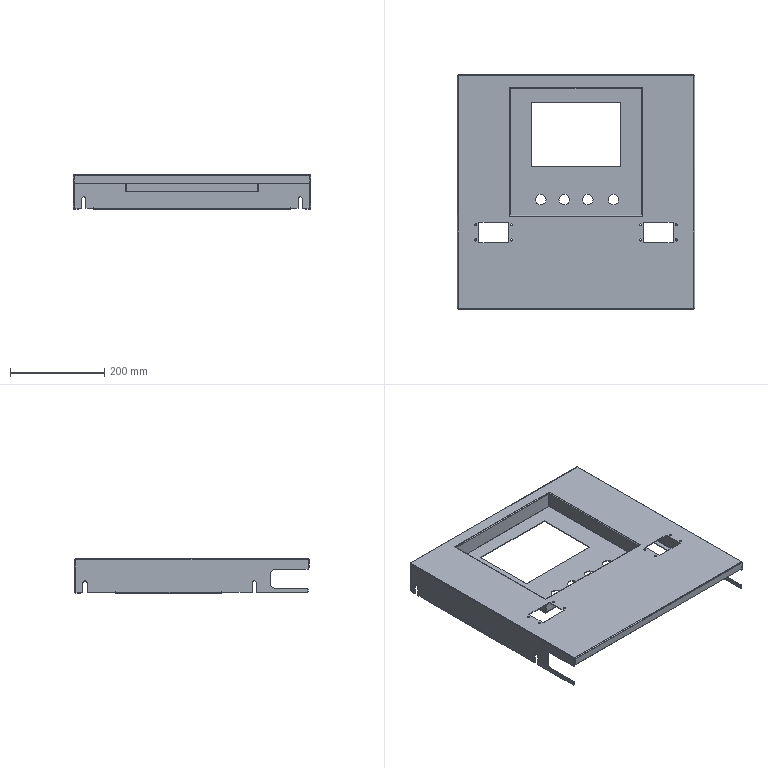Part | SolidWorks | features BaseBody 2 | 2 solids | 216 faces | box 505 x 498 x 73 mm | volume 552727 mm3 | plane 128 | cylinder 72 | spline 16 | commonest cylinder face diameters 4.5 x16 9 x12 1.473 x11 4.473 x11 6 x10 22.5 x8